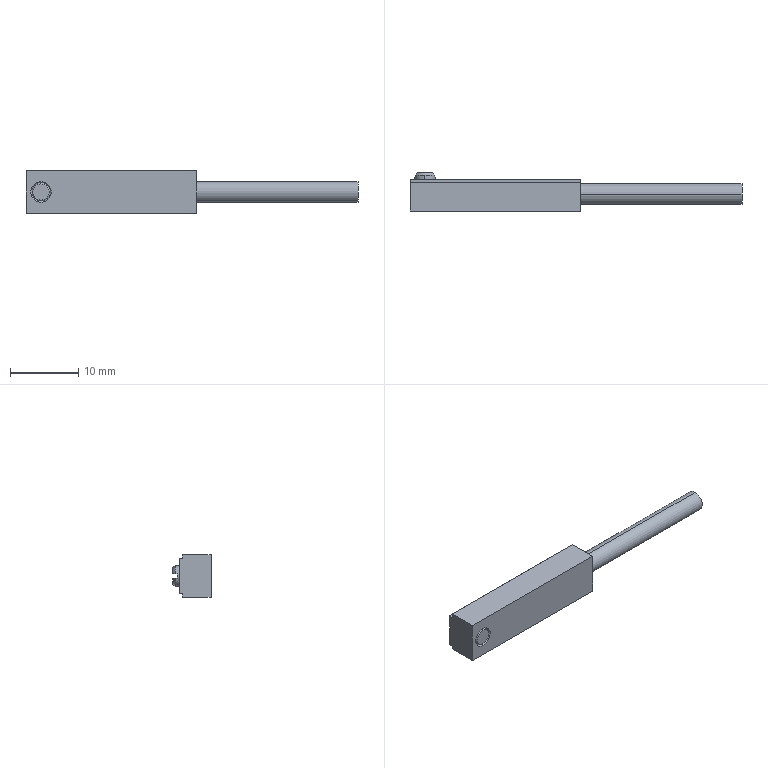Part | SolidWorks | features BaseBody 1 | 1 solid | 28 faces | box 48.8 x 5.6 x 6.3 mm | volume 899.301 mm3 | plane 17 | cone 7 | cylinder 4 | commonest cylinder face diameters 3 x4
STEP:
#1=CARTESIAN_POINT('',(0.7414,5.,-0.35));
#2=VERTEX_POINT('',#1);
#3=CARTESIAN_POINT('',(3.659,5.,-0.35));
#4=VERTEX_POINT('',#3);
#5=CARTESIAN_POINT('',(0.,5.,-0.35));
#6=DIRECTION('',(1.,0.,0.));
#7=VECTOR('',#6,1000.);
#8=LINE('',#5,#7);
#9=EDGE_CURVE('',#2,#4,#8,.T.);
#10=ORIENTED_EDGE('',*,*,#9,.F.);
#11=CARTESIAN_POINT('',(0.7414,5.,0.35));
#12=VERTEX_POINT('',#11);
#13=CARTESIAN_POINT('',(2.2,5.,0.));
#14=DIRECTION('',(0.,1.,0.));
#15=DIRECTION('',(0.,0.,1.));
#16=AXIS2_PLACEMENT_3D('',#13,#14,#15);
#17=CIRCLE('',#16,1.5);
#18=EDGE_CURVE('',#2,#12,#17,.T.);
#19=ORIENTED_EDGE('',*,*,#18,.T.);
#20=CARTESIAN_POINT('',(3.659,5.,0.35));
#21=VERTEX_POINT('',#20);
#22=CARTESIAN_POINT('',(0.,5.,0.35));
#23=DIRECTION('',(1.,0.,0.));
#24=VECTOR('',#23,1000.);
#25=LINE('',#22,#24);
#26=EDGE_CURVE('',#12,#21,#25,.T.);
#27=ORIENTED_EDGE('',*,*,#26,.T.);
#28=CARTESIAN_POINT('',(2.2,5.,0.));
#29=DIRECTION('',(0.,1.,0.));
#30=DIRECTION('',(0.,0.,1.));
#31=AXIS2_PLACEMENT_3D('',#28,#29,#30);
#32=CIRCLE('',#31,1.5);
#33=EDGE_CURVE('',#21,#4,#32,.T.);
#34=ORIENTED_EDGE('',*,*,#33,.T.);
#35=EDGE_LOOP('',(#10,#19,#27,#34));
#36=FACE_OUTER_BOUND('',#35,.T.);
#37=CARTESIAN_POINT('',(0.7,5.,0.35));
#38=DIRECTION('',(0.,1.,0.));
#39=DIRECTION('',(1.,0.,0.));
#40=AXIS2_PLACEMENT_3D('',#37,#38,#39);
#41=PLANE('',#40);
#42=ADVANCED_FACE('',(#36),#41,.T.);
#43=CARTESIAN_POINT('',(3.659,5.294,-0.35));
#44=VERTEX_POINT('',#43);
#45=CARTESIAN_POINT('',(3.341,5.6,-0.35));
#46=VERTEX_POINT('',#45);
#47=CARTESIAN_POINT('',(3.659,5.294,-0.35));
#48=CARTESIAN_POINT('',(3.553,5.396,-0.35));
#49=CARTESIAN_POINT('',(3.447,5.498,-0.35));
#50=CARTESIAN_POINT('',(3.341,5.6,-0.35));
#51=B_SPLINE_CURVE_WITH_KNOTS('',3,(#47,#48,#49,#50),.UNSPECIFIED.,.F.,.F.,(4,4),(0.,0.0004414),.UNSPECIFIED.);
#52=EDGE_CURVE('',#44,#46,#51,.T.);
#53=ORIENTED_EDGE('',*,*,#52,.T.);
#54=CARTESIAN_POINT('',(1.059,5.6,-0.35));
#55=VERTEX_POINT('',#54);
#56=CARTESIAN_POINT('',(2.2,5.6,-0.35));
#57=DIRECTION('',(-1.,0.,0.));
#58=VECTOR('',#57,1000.);
#59=LINE('',#56,#58);
#60=EDGE_CURVE('',#46,#55,#59,.T.);
#61=ORIENTED_EDGE('',*,*,#60,.T.);
#62=CARTESIAN_POINT('',(0.7414,5.294,-0.35));
#63=VERTEX_POINT('',#62);
#64=CARTESIAN_POINT('',(1.059,5.6,-0.35));
#65=CARTESIAN_POINT('',(0.9526,5.498,-0.35));
#66=CARTESIAN_POINT('',(0.8469,5.396,-0.35));
#67=CARTESIAN_POINT('',(0.7414,5.294,-0.35));
#68=B_SPLINE_CURVE_WITH_KNOTS('',3,(#64,#65,#66,#67),.UNSPECIFIED.,.F.,.F.,(4,4),(0.,0.0004414),.UNSPECIFIED.);
#69=EDGE_CURVE('',#55,#63,#68,.T.);
#70=ORIENTED_EDGE('',*,*,#69,.T.);
#71=CARTESIAN_POINT('',(0.7414,0.,-0.35));
#72=DIRECTION('',(0.,-1.,0.));
#73=VECTOR('',#72,1000.);
#74=LINE('',#71,#73);
#75=EDGE_CURVE('',#63,#2,#74,.T.);
#76=ORIENTED_EDGE('',*,*,#75,.T.);
#77=ORIENTED_EDGE('',*,*,#9,.T.);
#78=CARTESIAN_POINT('',(3.659,0.,-0.35));
#79=DIRECTION('',(0.,1.,0.));
#80=VECTOR('',#79,1000.);
#81=LINE('',#78,#80);
#82=EDGE_CURVE('',#4,#44,#81,.T.);
#83=ORIENTED_EDGE('',*,*,#82,.T.);
#84=EDGE_LOOP('',(#53,#61,#70,#76,#77,#83));
#85=FACE_OUTER_BOUND('',#84,.T.);
#86=CARTESIAN_POINT('',(0.,0.,-0.35));
#87=DIRECTION('',(0.,0.,1.));
#88=DIRECTION('',(1.,0.,0.));
#89=AXIS2_PLACEMENT_3D('',#86,#87,#88);
#90=PLANE('',#89);
#91=ADVANCED_FACE('',(#85),#90,.T.);
#92=CARTESIAN_POINT('',(3.659,5.294,0.35));
#93=VERTEX_POINT('',#92);
#94=CARTESIAN_POINT('',(3.341,5.6,0.35));
#95=VERTEX_POINT('',#94);
#96=CARTESIAN_POINT('',(3.659,5.294,0.35));
#97=CARTESIAN_POINT('',(3.553,5.396,0.35));
#98=CARTESIAN_POINT('',(3.447,5.498,0.35));
#99=CARTESIAN_POINT('',(3.341,5.6,0.35));
#100=B_SPLINE_CURVE_WITH_KNOTS('',3,(#96,#97,#98,#99),.UNSPECIFIED.,.F.,.F.,(4,4),(0.,0.0004414),.UNSPECIFIED.);
#101=EDGE_CURVE('',#93,#95,#100,.T.);
#102=ORIENTED_EDGE('',*,*,#101,.F.);
#103=CARTESIAN_POINT('',(3.659,0.,0.35));
#104=DIRECTION('',(0.,1.,0.));
#105=VECTOR('',#104,1000.);
#106=LINE('',#103,#105);
#107=EDGE_CURVE('',#21,#93,#106,.T.);
#108=ORIENTED_EDGE('',*,*,#107,.F.);
#109=ORIENTED_EDGE('',*,*,#26,.F.);
#110=CARTESIAN_POINT('',(0.7414,5.294,0.35));
#111=VERTEX_POINT('',#110);
#112=CARTESIAN_POINT('',(0.7414,0.,0.35));
#113=DIRECTION('',(0.,-1.,0.));
#114=VECTOR('',#113,1000.);
#115=LINE('',#112,#114);
#116=EDGE_CURVE('',#111,#12,#115,.T.);
#117=ORIENTED_EDGE('',*,*,#116,.F.);
#118=CARTESIAN_POINT('',(1.059,5.6,0.35));
#119=VERTEX_POINT('',#118);
#120=CARTESIAN_POINT('',(1.059,5.6,0.35));
#121=CARTESIAN_POINT('',(0.9526,5.498,0.35));
#122=CARTESIAN_POINT('',(0.8469,5.396,0.35));
#123=CARTESIAN_POINT('',(0.7414,5.294,0.35));
#124=B_SPLINE_CURVE_WITH_KNOTS('',3,(#120,#121,#122,#123),.UNSPECIFIED.,.F.,.F.,(4,4),(0.,0.0004414),.UNSPECIFIED.);
#125=EDGE_CURVE('',#119,#111,#124,.T.);
#126=ORIENTED_EDGE('',*,*,#125,.F.);
#127=CARTESIAN_POINT('',(2.2,5.6,0.35));
#128=DIRECTION('',(1.,0.,0.));
#129=VECTOR('',#128,1000.);
#130=LINE('',#127,#129);
#131=EDGE_CURVE('',#119,#95,#130,.T.);
#132=ORIENTED_EDGE('',*,*,#131,.T.);
#133=EDGE_LOOP('',(#102,#108,#109,#117,#126,#132));
#134=FACE_OUTER_BOUND('',#133,.T.);
#135=CARTESIAN_POINT('',(0.,0.,0.35));
#136=DIRECTION('',(0.,0.,1.));
#137=DIRECTION('',(1.,0.,0.));
#138=AXIS2_PLACEMENT_3D('',#135,#136,#137);
#139=PLANE('',#138);
#140=ADVANCED_FACE('',(#134),#139,.F.);
#141=CARTESIAN_POINT('',(2.2,0.,1.194));
#142=VERTEX_POINT('',#141);
#143=CARTESIAN_POINT('',(2.2,0.,-1.194));
#144=VERTEX_POINT('',#143);
#145=CARTESIAN_POINT('',(2.2,0.,0.));
#146=DIRECTION('',(0.,1.,0.));
#147=DIRECTION('',(0.,0.,1.));
#148=AXIS2_PLACEMENT_3D('',#145,#146,#147);
#149=CIRCLE('',#148,1.194);
#150=EDGE_CURVE('',#142,#144,#149,.T.);
#151=ORIENTED_EDGE('',*,*,#150,.F.);
#152=CARTESIAN_POINT('',(2.2,0.,0.));
#153=DIRECTION('',(0.,1.,0.));
#154=DIRECTION('',(0.,0.,1.));
#155=AXIS2_PLACEMENT_3D('',#152,#153,#154);
#156=CIRCLE('',#155,1.194);
#157=EDGE_CURVE('',#144,#142,#156,.T.);
#158=ORIENTED_EDGE('',*,*,#157,.F.);
#159=EDGE_LOOP('',(#151,#158));
#160=FACE_OUTER_BOUND('',#159,.T.);
#161=CARTESIAN_POINT('',(2.2,0.,-1.194));
#162=DIRECTION('',(0.,1.,0.));
#163=DIRECTION('',(1.,0.,0.));
#164=AXIS2_PLACEMENT_3D('',#161,#162,#163);
#165=PLANE('',#164);
#166=ADVANCED_FACE('',(#160),#165,.F.);
#167=CARTESIAN_POINT('',(2.2,5.6,-1.193));
#168=VERTEX_POINT('',#167);
#169=CARTESIAN_POINT('',(2.2,5.6,0.));
#170=DIRECTION('',(0.,-1.,0.));
#171=DIRECTION('',(0.,0.,-1.));
#172=AXIS2_PLACEMENT_3D('',#169,#170,#171);
#173=CIRCLE('',#172,1.193);
#174=EDGE_CURVE('',#55,#168,#173,.T.);
#175=ORIENTED_EDGE('',*,*,#174,.F.);
#176=ORIENTED_EDGE('',*,*,#60,.F.);
#177=CARTESIAN_POINT('',(2.2,5.6,0.));
#178=DIRECTION('',(0.,-1.,0.));
#179=DIRECTION('',(0.,0.,-1.));
#180=AXIS2_PLACEMENT_3D('',#177,#178,#179);
#181=CIRCLE('',#180,1.193);
#182=EDGE_CURVE('',#168,#46,#181,.T.);
#183=ORIENTED_EDGE('',*,*,#182,.F.);
#184=EDGE_LOOP('',(#175,#176,#183));
#185=FACE_OUTER_BOUND('',#184,.T.);
#186=CARTESIAN_POINT('',(2.2,5.6,0.));
#187=DIRECTION('',(0.,-1.,0.));
#188=DIRECTION('',(0.,0.,-1.));
#189=AXIS2_PLACEMENT_3D('',#186,#187,#188);
#190=PLANE('',#189);
#191=ADVANCED_FACE('',(#185),#190,.F.);
#192=ORIENTED_EDGE('',*,*,#131,.F.);
#193=CARTESIAN_POINT('',(2.2,5.6,0.));
#194=DIRECTION('',(0.,-1.,0.));
#195=DIRECTION('',(0.,0.,-1.));
#196=AXIS2_PLACEMENT_3D('',#193,#194,#195);
#197=CIRCLE('',#196,1.193);
#198=EDGE_CURVE('',#95,#119,#197,.T.);
#199=ORIENTED_EDGE('',*,*,#198,.F.);
#200=EDGE_LOOP('',(#192,#199));
#201=FACE_OUTER_BOUND('',#200,.T.);
#202=CARTESIAN_POINT('',(2.2,5.6,0.));
#203=DIRECTION('',(0.,-1.,0.));
#204=DIRECTION('',(0.,0.,-1.));
#205=AXIS2_PLACEMENT_3D('',#202,#203,#204);
#206=PLANE('',#205);
#207=ADVANCED_FACE('',(#201),#206,.F.);
#208=CARTESIAN_POINT('',(2.2,0.1532,-1.347));
#209=VERTEX_POINT('',#208);
#210=CARTESIAN_POINT('',(2.2,0.1532,-1.347));
#211=DIRECTION('',(0.,0.7071,-0.7071));
#212=VECTOR('',#211,1000.);
#213=LINE('',#210,#212);
#214=EDGE_CURVE('',#144,#209,#213,.T.);
#215=ORIENTED_EDGE('',*,*,#214,.F.);
#216=ORIENTED_EDGE('',*,*,#157,.T.);
#217=CARTESIAN_POINT('',(2.2,0.1532,1.347));
#218=VERTEX_POINT('',#217);
#219=CARTESIAN_POINT('',(2.2,0.1532,1.347));
#220=DIRECTION('',(0.,0.7071,0.7071));
#221=VECTOR('',#220,1000.);
#222=LINE('',#219,#221);
#223=EDGE_CURVE('',#142,#218,#222,.T.);
#224=ORIENTED_EDGE('',*,*,#223,.T.);
#225=CARTESIAN_POINT('',(2.2,0.1532,0.));
#226=DIRECTION('',(0.,-1.,0.));
#227=DIRECTION('',(0.,0.,-1.));
#228=AXIS2_PLACEMENT_3D('',#225,#226,#227);
#229=CIRCLE('',#228,1.347);
#230=EDGE_CURVE('',#218,#209,#229,.T.);
#231=ORIENTED_EDGE('',*,*,#230,.T.);
#232=EDGE_LOOP('',(#215,#216,#224,#231));
#233=FACE_OUTER_BOUND('',#232,.T.);
#234=CARTESIAN_POINT('',(2.2,0.1532,0.));
#235=DIRECTION('',(0.,1.,0.));
#236=DIRECTION('',(0.,0.,1.));
#237=AXIS2_PLACEMENT_3D('',#234,#235,#236);
#238=CONICAL_SURFACE('',#237,1.347,0.7854);
#239=ADVANCED_FACE('',(#233),#238,.T.);
#240=CARTESIAN_POINT('',(2.2,5.293,-1.5));
#241=VERTEX_POINT('',#240);
#242=CARTESIAN_POINT('',(2.2,5.294,-1.5));
#243=DIRECTION('',(0.,-0.7071,-0.7071));
#244=VECTOR('',#243,1000.);
#245=LINE('',#242,#244);
#246=EDGE_CURVE('',#168,#241,#245,.T.);
#247=ORIENTED_EDGE('',*,*,#246,.F.);
#248=ORIENTED_EDGE('',*,*,#182,.T.);
#249=ORIENTED_EDGE('',*,*,#52,.F.);
#250=CARTESIAN_POINT('',(2.2,5.293,0.));
#251=DIRECTION('',(0.,-1.,0.));
#252=DIRECTION('',(0.,0.,1.));
#253=AXIS2_PLACEMENT_3D('',#250,#251,#252);
#254=CIRCLE('',#253,1.5);
#255=EDGE_CURVE('',#241,#44,#254,.T.);
#256=ORIENTED_EDGE('',*,*,#255,.F.);
#257=EDGE_LOOP('',(#247,#248,#249,#256));
#258=FACE_OUTER_BOUND('',#257,.T.);
#259=CARTESIAN_POINT('',(2.2,5.294,0.));
#260=DIRECTION('',(0.,-1.,0.));
#261=DIRECTION('',(0.,0.,-1.));
#262=AXIS2_PLACEMENT_3D('',#259,#260,#261);
#263=CONICAL_SURFACE('',#262,1.5,0.7854);
#264=ADVANCED_FACE('',(#258),#263,.T.);
#265=ORIENTED_EDGE('',*,*,#198,.T.);
#266=ORIENTED_EDGE('',*,*,#125,.T.);
#267=CARTESIAN_POINT('',(2.2,5.293,1.5));
#268=VERTEX_POINT('',#267);
#269=CARTESIAN_POINT('',(2.2,5.293,0.));
#270=DIRECTION('',(0.,-1.,0.));
#271=DIRECTION('',(0.,0.,1.));
#272=AXIS2_PLACEMENT_3D('',#269,#270,#271);
#273=CIRCLE('',#272,1.5);
#274=EDGE_CURVE('',#268,#111,#273,.T.);
#275=ORIENTED_EDGE('',*,*,#274,.F.);
#276=CARTESIAN_POINT('',(2.2,5.293,0.));
#277=DIRECTION('',(0.,-1.,0.));
#278=DIRECTION('',(0.,0.,1.));
#279=AXIS2_PLACEMENT_3D('',#276,#277,#278);
#280=CIRCLE('',#279,1.5);
#281=EDGE_CURVE('',#93,#268,#280,.T.);
#282=ORIENTED_EDGE('',*,*,#281,.F.);
#283=ORIENTED_EDGE('',*,*,#101,.T.);
#284=EDGE_LOOP('',(#265,#266,#275,#282,#283));
#285=FACE_OUTER_BOUND('',#284,.T.);
#286=CARTESIAN_POINT('',(2.2,5.294,0.));
#287=DIRECTION('',(0.,-1.,0.));
#288=DIRECTION('',(0.,0.,-1.));
#289=AXIS2_PLACEMENT_3D('',#286,#287,#288);
#290=CONICAL_SURFACE('',#289,1.5,0.7854);
#291=ADVANCED_FACE('',(#285),#290,.T.);
#292=CARTESIAN_POINT('',(0.,4.2,3.15));
#293=VERTEX_POINT('',#292);
#294=CARTESIAN_POINT('',(25.,4.2,3.15));
#295=VERTEX_POINT('',#294);
#296=CARTESIAN_POINT('',(25.,4.2,3.15));
#297=DIRECTION('',(1.,0.,0.));
#298=VECTOR('',#297,1000.);
#299=LINE('',#296,#298);
#300=EDGE_CURVE('',#293,#295,#299,.T.);
#301=ORIENTED_EDGE('',*,*,#300,.T.);
#302=CARTESIAN_POINT('',(25.,4.2,2.6));
#303=VERTEX_POINT('',#302);
#304=CARTESIAN_POINT('',(25.,4.2,2.6));
#305=DIRECTION('',(0.,0.,1.));
#306=VECTOR('',#305,1000.);
#307=LINE('',#304,#306);
#308=EDGE_CURVE('',#303,#295,#307,.T.);
#309=ORIENTED_EDGE('',*,*,#308,.F.);
#310=CARTESIAN_POINT('',(0.,4.2,2.6));
#311=VERTEX_POINT('',#310);
#312=CARTESIAN_POINT('',(25.,4.2,2.6));
#313=DIRECTION('',(-1.,0.,0.));
#314=VECTOR('',#313,1000.);
#315=LINE('',#312,#314);
#316=EDGE_CURVE('',#303,#311,#315,.T.);
#317=ORIENTED_EDGE('',*,*,#316,.T.);
#318=CARTESIAN_POINT('',(0.,4.2,0.));
#319=DIRECTION('',(0.,0.,1.));
#320=VECTOR('',#319,1000.);
#321=LINE('',#318,#320);
#322=EDGE_CURVE('',#311,#293,#321,.T.);
#323=ORIENTED_EDGE('',*,*,#322,.T.);
#324=EDGE_LOOP('',(#301,#309,#317,#323));
#325=FACE_OUTER_BOUND('',#324,.T.);
#326=CARTESIAN_POINT('',(25.,4.2,2.6));
#327=DIRECTION('',(0.,-1.,0.));
#328=DIRECTION('',(0.,0.,-1.));
#329=AXIS2_PLACEMENT_3D('',#326,#327,#328);
#330=PLANE('',#329);
#331=ADVANCED_FACE('',(#325),#330,.F.);
#332=CARTESIAN_POINT('',(2.2,0.,1.5));
#333=VERTEX_POINT('',#332);
#334=CARTESIAN_POINT('',(2.2,0.,1.5));
#335=DIRECTION('',(0.,-0.7071,0.7071));
#336=VECTOR('',#335,1000.);
#337=LINE('',#334,#336);
#338=EDGE_CURVE('',#218,#333,#337,.T.);
#339=ORIENTED_EDGE('',*,*,#338,.F.);
#340=CARTESIAN_POINT('',(2.2,0.1532,0.));
#341=DIRECTION('',(0.,-1.,0.));
#342=DIRECTION('',(0.,0.,-1.));
#343=AXIS2_PLACEMENT_3D('',#340,#341,#342);
#344=CIRCLE('',#343,1.347);
#345=EDGE_CURVE('',#209,#218,#344,.T.);
#346=ORIENTED_EDGE('',*,*,#345,.F.);
#347=CARTESIAN_POINT('',(2.2,0.,-1.5));
#348=VERTEX_POINT('',#347);
#349=CARTESIAN_POINT('',(2.2,0.,-1.5));
#350=DIRECTION('',(0.,-0.7071,-0.7071));
#351=VECTOR('',#350,1000.);
#352=LINE('',#349,#351);
#353=EDGE_CURVE('',#209,#348,#352,.T.);
#354=ORIENTED_EDGE('',*,*,#353,.T.);
#355=CARTESIAN_POINT('',(2.2,0.,0.));
#356=DIRECTION('',(0.,-1.,0.));
#357=DIRECTION('',(0.,0.,-1.));
#358=AXIS2_PLACEMENT_3D('',#355,#356,#357);
#359=CIRCLE('',#358,1.5);
#360=EDGE_CURVE('',#348,#333,#359,.T.);
#361=ORIENTED_EDGE('',*,*,#360,.T.);
#362=EDGE_LOOP('',(#339,#346,#354,#361));
#363=FACE_OUTER_BOUND('',#362,.T.);
#364=CARTESIAN_POINT('',(2.2,0.,0.));
#365=DIRECTION('',(0.,-1.,0.));
#366=DIRECTION('',(0.,0.,-1.));
#367=AXIS2_PLACEMENT_3D('',#364,#365,#366);
#368=CONICAL_SURFACE('',#367,1.5,0.7854);
#369=ADVANCED_FACE('',(#363),#368,.F.);
#370=CARTESIAN_POINT('',(0.,4.2,-2.6));
#371=VERTEX_POINT('',#370);
#372=CARTESIAN_POINT('',(25.,4.2,-2.6));
#373=VERTEX_POINT('',#372);
#374=CARTESIAN_POINT('',(25.,4.2,-2.6));
#375=DIRECTION('',(1.,0.,0.));
#376=VECTOR('',#375,1000.);
#377=LINE('',#374,#376);
#378=EDGE_CURVE('',#371,#373,#377,.T.);
#379=ORIENTED_EDGE('',*,*,#378,.T.);
#380=CARTESIAN_POINT('',(25.,4.2,-3.15));
#381=VERTEX_POINT('',#380);
#382=CARTESIAN_POINT('',(25.,4.2,-3.15));
#383=DIRECTION('',(0.,0.,1.));
#384=VECTOR('',#383,1000.);
#385=LINE('',#382,#384);
#386=EDGE_CURVE('',#381,#373,#385,.T.);
#387=ORIENTED_EDGE('',*,*,#386,.F.);
#388=CARTESIAN_POINT('',(0.,4.2,-3.15));
#389=VERTEX_POINT('',#388);
#390=CARTESIAN_POINT('',(25.,4.2,-3.15));
#391=DIRECTION('',(-1.,0.,0.));
#392=VECTOR('',#391,1000.);
#393=LINE('',#390,#392);
#394=EDGE_CURVE('',#381,#389,#393,.T.);
#395=ORIENTED_EDGE('',*,*,#394,.T.);
#396=CARTESIAN_POINT('',(0.,4.2,0.));
#397=DIRECTION('',(0.,0.,1.));
#398=VECTOR('',#397,1000.);
#399=LINE('',#396,#398);
#400=EDGE_CURVE('',#389,#371,#399,.T.);
#401=ORIENTED_EDGE('',*,*,#400,.T.);
#402=EDGE_LOOP('',(#379,#387,#395,#401));
#403=FACE_OUTER_BOUND('',#402,.T.);
#404=CARTESIAN_POINT('',(25.,4.2,-3.15));
#405=DIRECTION('',(0.,-1.,0.));
#406=DIRECTION('',(0.,0.,-1.));
#407=AXIS2_PLACEMENT_3D('',#404,#405,#406);
#408=PLANE('',#407);
#409=ADVANCED_FACE('',(#403),#408,.F.);
#410=CARTESIAN_POINT('',(2.2,4.7,-1.5));
#411=VERTEX_POINT('',#410);
#412=CARTESIAN_POINT('',(2.2,0.,-1.5));
#413=DIRECTION('',(0.,1.,0.));
#414=VECTOR('',#413,1000.);
#415=LINE('',#412,#414);
#416=EDGE_CURVE('',#411,#241,#415,.T.);
#417=ORIENTED_EDGE('',*,*,#416,.F.);
#418=CARTESIAN_POINT('',(2.2,4.7,1.5));
#419=VERTEX_POINT('',#418);
#420=CARTESIAN_POINT('',(2.2,4.7,0.));
#421=DIRECTION('',(0.,1.,0.));
#422=DIRECTION('',(0.,0.,1.));
#423=AXIS2_PLACEMENT_3D('',#420,#421,#422);
#424=CIRCLE('',#423,1.5);
#425=EDGE_CURVE('',#411,#419,#424,.T.);
#426=ORIENTED_EDGE('',*,*,#425,.T.);
#427=CARTESIAN_POINT('',(2.2,0.,1.5));
#428=DIRECTION('',(0.,1.,0.));
#429=VECTOR('',#428,1000.);
#430=LINE('',#427,#429);
#431=EDGE_CURVE('',#419,#268,#430,.T.);
#432=ORIENTED_EDGE('',*,*,#431,.T.);
#433=ORIENTED_EDGE('',*,*,#274,.T.);
#434=ORIENTED_EDGE('',*,*,#116,.T.);
#435=ORIENTED_EDGE('',*,*,#18,.F.);
#436=ORIENTED_EDGE('',*,*,#75,.F.);
#437=CARTESIAN_POINT('',(2.2,5.293,0.));
#438=DIRECTION('',(0.,-1.,0.));
#439=DIRECTION('',(0.,0.,1.));
#440=AXIS2_PLACEMENT_3D('',#437,#438,#439);
#441=CIRCLE('',#440,1.5);
#442=EDGE_CURVE('',#63,#241,#441,.T.);
#443=ORIENTED_EDGE('',*,*,#442,.T.);
#444=EDGE_LOOP('',(#417,#426,#432,#433,#434,#435,#436,#443));
#445=FACE_OUTER_BOUND('',#444,.T.);
#446=CARTESIAN_POINT('',(2.2,0.,0.));
#447=DIRECTION('',(0.,1.,0.));
#448=DIRECTION('',(0.,0.,1.));
#449=AXIS2_PLACEMENT_3D('',#446,#447,#448);
#450=CYLINDRICAL_SURFACE('',#449,1.5);
#451=ADVANCED_FACE('',(#445),#450,.T.);
#452=CARTESIAN_POINT('',(0.,4.7,-2.6));
#453=VERTEX_POINT('',#452);
#454=CARTESIAN_POINT('',(25.,4.7,-2.6));
#455=VERTEX_POINT('',#454);
#456=CARTESIAN_POINT('',(25.,4.7,-2.6));
#457=DIRECTION('',(1.,0.,0.));
#458=VECTOR('',#457,1000.);
#459=LINE('',#456,#458);
#460=EDGE_CURVE('',#453,#455,#459,.T.);
#461=ORIENTED_EDGE('',*,*,#460,.T.);
#462=CARTESIAN_POINT('',(25.,4.2,-2.6));
#463=DIRECTION('',(0.,1.,0.));
#464=VECTOR('',#463,1000.);
#465=LINE('',#462,#464);
#466=EDGE_CURVE('',#373,#455,#465,.T.);
#467=ORIENTED_EDGE('',*,*,#466,.F.);
#468=ORIENTED_EDGE('',*,*,#378,.F.);
#469=CARTESIAN_POINT('',(0.,0.,-2.6));
#470=DIRECTION('',(0.,1.,0.));
#471=VECTOR('',#470,1000.);
#472=LINE('',#469,#471);
#473=EDGE_CURVE('',#371,#453,#472,.T.);
#474=ORIENTED_EDGE('',*,*,#473,.T.);
#475=EDGE_LOOP('',(#461,#467,#468,#474));
#476=FACE_OUTER_BOUND('',#475,.T.);
#477=CARTESIAN_POINT('',(25.,4.2,-2.6));
#478=DIRECTION('',(0.,0.,1.));
#479=DIRECTION('',(1.,0.,0.));
#480=AXIS2_PLACEMENT_3D('',#477,#478,#479);
#481=PLANE('',#480);
#482=ADVANCED_FACE('',(#476),#481,.F.);
#483=ORIENTED_EDGE('',*,*,#316,.F.);
#484=CARTESIAN_POINT('',(25.,4.7,2.6));
#485=VERTEX_POINT('',#484);
#486=CARTESIAN_POINT('',(25.,4.7,2.6));
#487=DIRECTION('',(0.,-1.,0.));
#488=VECTOR('',#487,1000.);
#489=LINE('',#486,#488);
#490=EDGE_CURVE('',#485,#303,#489,.T.);
#491=ORIENTED_EDGE('',*,*,#490,.F.);
#492=CARTESIAN_POINT('',(0.,4.7,2.6));
#493=VERTEX_POINT('',#492);
#494=CARTESIAN_POINT('',(25.,4.7,2.6));
#495=DIRECTION('',(-1.,0.,0.));
#496=VECTOR('',#495,1000.);
#497=LINE('',#494,#496);
#498=EDGE_CURVE('',#485,#493,#497,.T.);
#499=ORIENTED_EDGE('',*,*,#498,.T.);
#500=CARTESIAN_POINT('',(0.,0.,2.6));
#501=DIRECTION('',(0.,-1.,0.));
#502=VECTOR('',#501,1000.);
#503=LINE('',#500,#502);
#504=EDGE_CURVE('',#493,#311,#503,.T.);
#505=ORIENTED_EDGE('',*,*,#504,.T.);
#506=EDGE_LOOP('',(#483,#491,#499,#505));
#507=FACE_OUTER_BOUND('',#506,.T.);
#508=CARTESIAN_POINT('',(25.,4.7,2.6));
#509=DIRECTION('',(0.,0.,-1.));
#510=DIRECTION('',(0.,-1.,0.));
#511=AXIS2_PLACEMENT_3D('',#508,#509,#510);
#512=PLANE('',#511);
#513=ADVANCED_FACE('',(#507),#512,.F.);
#514=ORIENTED_EDGE('',*,*,#322,.F.);
#515=ORIENTED_EDGE('',*,*,#504,.F.);
#516=CARTESIAN_POINT('',(0.,4.7,-2.6));
#517=DIRECTION('',(0.,0.,-1.));
#518=VECTOR('',#517,1000.);
#519=LINE('',#516,#518);
#520=EDGE_CURVE('',#493,#453,#519,.T.);
#521=ORIENTED_EDGE('',*,*,#520,.T.);
#522=ORIENTED_EDGE('',*,*,#473,.F.);
#523=ORIENTED_EDGE('',*,*,#400,.F.);
#524=CARTESIAN_POINT('',(0.,0.,-3.15));
#525=VERTEX_POINT('',#524);
#526=CARTESIAN_POINT('',(0.,0.,-3.15));
#527=DIRECTION('',(0.,-1.,0.));
#528=VECTOR('',#527,1000.);
#529=LINE('',#526,#528);
#530=EDGE_CURVE('',#389,#525,#529,.T.);
#531=ORIENTED_EDGE('',*,*,#530,.T.);
#532=CARTESIAN_POINT('',(0.,0.,3.15));
#533=VERTEX_POINT('',#532);
#534=CARTESIAN_POINT('',(0.,0.,3.15));
#535=DIRECTION('',(0.,0.,1.));
#536=VECTOR('',#535,1000.);
#537=LINE('',#534,#536);
#538=EDGE_CURVE('',#525,#533,#537,.T.);
#539=ORIENTED_EDGE('',*,*,#538,.T.);
#540=CARTESIAN_POINT('',(0.,4.2,3.15));
#541=DIRECTION('',(0.,1.,0.));
#542=VECTOR('',#541,1000.);
#543=LINE('',#540,#542);
#544=EDGE_CURVE('',#533,#293,#543,.T.);
#545=ORIENTED_EDGE('',*,*,#544,.T.);
#546=EDGE_LOOP('',(#514,#515,#521,#522,#523,#531,#539,#545));
#547=FACE_OUTER_BOUND('',#546,.T.);
#548=CARTESIAN_POINT('',(0.,0.,0.));
#549=DIRECTION('',(1.,0.,0.));
#550=DIRECTION('',(0.,1.,0.));
#551=AXIS2_PLACEMENT_3D('',#548,#549,#550);
#552=PLANE('',#551);
#553=ADVANCED_FACE('',(#547),#552,.F.);
#554=CARTESIAN_POINT('',(25.,0.,3.15));
#555=VERTEX_POINT('',#554);
#556=CARTESIAN_POINT('',(25.,0.,3.15));
#557=DIRECTION('',(1.,0.,0.));
#558=VECTOR('',#557,1000.);
#559=LINE('',#556,#558);
#560=EDGE_CURVE('',#533,#555,#559,.T.);
#561=ORIENTED_EDGE('',*,*,#560,.T.);
#562=CARTESIAN_POINT('',(25.,0.,3.15));
#563=DIRECTION('',(0.,-1.,0.));
#564=VECTOR('',#563,1000.);
#565=LINE('',#562,#564);
#566=EDGE_CURVE('',#295,#555,#565,.T.);
#567=ORIENTED_EDGE('',*,*,#566,.F.);
#568=ORIENTED_EDGE('',*,*,#300,.F.);
#569=ORIENTED_EDGE('',*,*,#544,.F.);
#570=EDGE_LOOP('',(#561,#567,#568,#569));
#571=FACE_OUTER_BOUND('',#570,.T.);
#572=CARTESIAN_POINT('',(25.,4.2,3.15));
#573=DIRECTION('',(0.,0.,-1.));
#574=DIRECTION('',(0.,-1.,0.));
#575=AXIS2_PLACEMENT_3D('',#572,#573,#574);
#576=PLANE('',#575);
#577=ADVANCED_FACE('',(#571),#576,.F.);
#578=ORIENTED_EDGE('',*,*,#360,.F.);
#579=CARTESIAN_POINT('',(2.2,0.,0.));
#580=DIRECTION('',(0.,-1.,0.));
#581=DIRECTION('',(0.,0.,-1.));
#582=AXIS2_PLACEMENT_3D('',#579,#580,#581);
#583=CIRCLE('',#582,1.5);
#584=EDGE_CURVE('',#333,#348,#583,.T.);
#585=ORIENTED_EDGE('',*,*,#584,.F.);
#586=EDGE_LOOP('',(#578,#585));
#587=FACE_BOUND('',#586,.T.);
#588=CARTESIAN_POINT('',(25.,0.,-3.15));
#589=VERTEX_POINT('',#588);
#590=CARTESIAN_POINT('',(25.,0.,-3.15));
#591=DIRECTION('',(1.,0.,0.));
#592=VECTOR('',#591,1000.);
#593=LINE('',#590,#592);
#594=EDGE_CURVE('',#525,#589,#593,.T.);
#595=ORIENTED_EDGE('',*,*,#594,.T.);
#596=CARTESIAN_POINT('',(25.,0.,0.));
#597=DIRECTION('',(0.,0.,-1.));
#598=VECTOR('',#597,1000.);
#599=LINE('',#596,#598);
#600=EDGE_CURVE('',#555,#589,#599,.T.);
#601=ORIENTED_EDGE('',*,*,#600,.F.);
#602=ORIENTED_EDGE('',*,*,#560,.F.);
#603=ORIENTED_EDGE('',*,*,#538,.F.);
#604=EDGE_LOOP('',(#595,#601,#602,#603));
#605=FACE_OUTER_BOUND('',#604,.T.);
#606=CARTESIAN_POINT('',(25.,0.,3.15));
#607=DIRECTION('',(0.,1.,0.));
#608=DIRECTION('',(1.,0.,0.));
#609=AXIS2_PLACEMENT_3D('',#606,#607,#608);
#610=PLANE('',#609);
#611=ADVANCED_FACE('',(#587,#605),#610,.F.);
#612=ORIENTED_EDGE('',*,*,#394,.F.);
#613=CARTESIAN_POINT('',(25.,0.,-3.15));
#614=DIRECTION('',(0.,1.,0.));
#615=VECTOR('',#614,1000.);
#616=LINE('',#613,#615);
#617=EDGE_CURVE('',#589,#381,#616,.T.);
#618=ORIENTED_EDGE('',*,*,#617,.F.);
#619=ORIENTED_EDGE('',*,*,#594,.F.);
#620=ORIENTED_EDGE('',*,*,#530,.F.);
#621=EDGE_LOOP('',(#612,#618,#619,#620));
#622=FACE_OUTER_BOUND('',#621,.T.);
#623=CARTESIAN_POINT('',(25.,0.,-3.15));
#624=DIRECTION('',(0.,0.,1.));
#625=DIRECTION('',(1.,0.,0.));
#626=AXIS2_PLACEMENT_3D('',#623,#624,#625);
#627=PLANE('',#626);
#628=ADVANCED_FACE('',(#622),#627,.F.);
#629=CARTESIAN_POINT('',(2.2,4.7,0.));
#630=DIRECTION('',(0.,1.,0.));
#631=DIRECTION('',(0.,0.,1.));
#632=AXIS2_PLACEMENT_3D('',#629,#630,#631);
#633=CIRCLE('',#632,1.5);
#634=EDGE_CURVE('',#419,#411,#633,.T.);
#635=ORIENTED_EDGE('',*,*,#634,.F.);
#636=ORIENTED_EDGE('',*,*,#425,.F.);
#637=EDGE_LOOP('',(#635,#636));
#638=FACE_BOUND('',#637,.T.);
#639=ORIENTED_EDGE('',*,*,#498,.F.);
#640=CARTESIAN_POINT('',(25.,4.7,0.));
#641=DIRECTION('',(0.,0.,1.));
#642=VECTOR('',#641,1000.);
#643=LINE('',#640,#642);
#644=EDGE_CURVE('',#455,#485,#643,.T.);
#645=ORIENTED_EDGE('',*,*,#644,.F.);
#646=ORIENTED_EDGE('',*,*,#460,.F.);
#647=ORIENTED_EDGE('',*,*,#520,.F.);
#648=EDGE_LOOP('',(#639,#645,#646,#647));
#649=FACE_OUTER_BOUND('',#648,.T.);
#650=CARTESIAN_POINT('',(25.,4.7,-2.6));
#651=DIRECTION('',(0.,-1.,0.));
#652=DIRECTION('',(0.,0.,-1.));
#653=AXIS2_PLACEMENT_3D('',#650,#651,#652);
#654=PLANE('',#653);
#655=ADVANCED_FACE('',(#638,#649),#654,.F.);
#656=CARTESIAN_POINT('',(25.,2.5,-1.5));
#657=VERTEX_POINT('',#656);
#658=CARTESIAN_POINT('',(25.,2.5,1.5));
#659=VERTEX_POINT('',#658);
#660=CARTESIAN_POINT('',(25.,2.5,0.));
#661=DIRECTION('',(1.,0.,0.));
#662=DIRECTION('',(0.,0.,-1.));
#663=AXIS2_PLACEMENT_3D('',#660,#661,#662);
#664=CIRCLE('',#663,1.5);
#665=EDGE_CURVE('',#657,#659,#664,.T.);
#666=ORIENTED_EDGE('',*,*,#665,.F.);
#667=CARTESIAN_POINT('',(25.,2.5,0.));
#668=DIRECTION('',(1.,0.,0.));
#669=DIRECTION('',(0.,0.,-1.));
#670=AXIS2_PLACEMENT_3D('',#667,#668,#669);
#671=CIRCLE('',#670,1.5);
#672=EDGE_CURVE('',#659,#657,#671,.T.);
#673=ORIENTED_EDGE('',*,*,#672,.F.);
#674=EDGE_LOOP('',(#666,#673));
#675=FACE_BOUND('',#674,.T.);
#676=ORIENTED_EDGE('',*,*,#490,.T.);
#677=ORIENTED_EDGE('',*,*,#308,.T.);
#678=ORIENTED_EDGE('',*,*,#566,.T.);
#679=ORIENTED_EDGE('',*,*,#600,.T.);
#680=ORIENTED_EDGE('',*,*,#617,.T.);
#681=ORIENTED_EDGE('',*,*,#386,.T.);
#682=ORIENTED_EDGE('',*,*,#466,.T.);
#683=ORIENTED_EDGE('',*,*,#644,.T.);
#684=EDGE_LOOP('',(#676,#677,#678,#679,#680,#681,#682,#683));
#685=FACE_OUTER_BOUND('',#684,.T.);
#686=CARTESIAN_POINT('',(25.,0.,0.));
#687=DIRECTION('',(1.,0.,0.));
#688=DIRECTION('',(0.,1.,0.));
#689=AXIS2_PLACEMENT_3D('',#686,#687,#688);
#690=PLANE('',#689);
#691=ADVANCED_FACE('',(#675,#685),#690,.T.);
#692=CARTESIAN_POINT('',(48.8,2.5,-1.5));
#693=VERTEX_POINT('',#692);
#694=CARTESIAN_POINT('',(48.8,2.5,1.5));
#695=VERTEX_POINT('',#694);
#696=CARTESIAN_POINT('',(48.8,2.5,0.));
#697=DIRECTION('',(-1.,0.,0.));
#698=DIRECTION('',(0.,0.,-1.));
#699=AXIS2_PLACEMENT_3D('',#696,#697,#698);
#700=CIRCLE('',#699,1.5);
#701=EDGE_CURVE('',#693,#695,#700,.T.);
#702=ORIENTED_EDGE('',*,*,#701,.F.);
#703=CARTESIAN_POINT('',(48.8,2.5,0.));
#704=DIRECTION('',(-1.,0.,0.));
#705=DIRECTION('',(0.,0.,-1.));
#706=AXIS2_PLACEMENT_3D('',#703,#704,#705);
#707=CIRCLE('',#706,1.5);
#708=EDGE_CURVE('',#695,#693,#707,.T.);
#709=ORIENTED_EDGE('',*,*,#708,.F.);
#710=EDGE_LOOP('',(#702,#709));
#711=FACE_OUTER_BOUND('',#710,.T.);
#712=CARTESIAN_POINT('',(48.8,2.5,0.));
#713=DIRECTION('',(1.,0.,0.));
#714=DIRECTION('',(0.,1.,0.));
#715=AXIS2_PLACEMENT_3D('',#712,#713,#714);
#716=PLANE('',#715);
#717=ADVANCED_FACE('',(#711),#716,.T.);
#718=CARTESIAN_POINT('',(48.8,2.5,1.5));
#719=DIRECTION('',(1.,0.,0.));
#720=VECTOR('',#719,1000.);
#721=LINE('',#718,#720);
#722=EDGE_CURVE('',#659,#695,#721,.T.);
#723=ORIENTED_EDGE('',*,*,#722,.F.);
#724=ORIENTED_EDGE('',*,*,#672,.T.);
#725=CARTESIAN_POINT('',(48.8,2.5,-1.5));
#726=DIRECTION('',(1.,0.,0.));
#727=VECTOR('',#726,1000.);
#728=LINE('',#725,#727);
#729=EDGE_CURVE('',#657,#693,#728,.T.);
#730=ORIENTED_EDGE('',*,*,#729,.T.);
#731=ORIENTED_EDGE('',*,*,#701,.T.);
#732=EDGE_LOOP('',(#723,#724,#730,#731));
#733=FACE_OUTER_BOUND('',#732,.T.);
#734=CARTESIAN_POINT('',(48.8,2.5,0.));
#735=DIRECTION('',(1.,0.,0.));
#736=DIRECTION('',(0.,0.,-1.));
#737=AXIS2_PLACEMENT_3D('',#734,#735,#736);
#738=CYLINDRICAL_SURFACE('',#737,1.5);
#739=ADVANCED_FACE('',(#733),#738,.T.);
#740=ORIENTED_EDGE('',*,*,#150,.T.);
#741=ORIENTED_EDGE('',*,*,#214,.T.);
#742=ORIENTED_EDGE('',*,*,#345,.T.);
#743=ORIENTED_EDGE('',*,*,#223,.F.);
#744=EDGE_LOOP('',(#740,#741,#742,#743));
#745=FACE_OUTER_BOUND('',#744,.T.);
#746=CARTESIAN_POINT('',(2.2,0.1532,0.));
#747=DIRECTION('',(0.,1.,0.));
#748=DIRECTION('',(0.,0.,1.));
#749=AXIS2_PLACEMENT_3D('',#746,#747,#748);
#750=CONICAL_SURFACE('',#749,1.347,0.7854);
#751=ADVANCED_FACE('',(#745),#750,.T.);
#752=ORIENTED_EDGE('',*,*,#174,.T.);
#753=ORIENTED_EDGE('',*,*,#246,.T.);
#754=ORIENTED_EDGE('',*,*,#442,.F.);
#755=ORIENTED_EDGE('',*,*,#69,.F.);
#756=EDGE_LOOP('',(#752,#753,#754,#755));
#757=FACE_OUTER_BOUND('',#756,.T.);
#758=CARTESIAN_POINT('',(2.2,5.294,0.));
#759=DIRECTION('',(0.,-1.,0.));
#760=DIRECTION('',(0.,0.,-1.));
#761=AXIS2_PLACEMENT_3D('',#758,#759,#760);
#762=CONICAL_SURFACE('',#761,1.5,0.7854);
#763=ADVANCED_FACE('',(#757),#762,.T.);
#764=ORIENTED_EDGE('',*,*,#230,.F.);
#765=ORIENTED_EDGE('',*,*,#338,.T.);
#766=ORIENTED_EDGE('',*,*,#584,.T.);
#767=ORIENTED_EDGE('',*,*,#353,.F.);
#768=EDGE_LOOP('',(#764,#765,#766,#767));
#769=FACE_OUTER_BOUND('',#768,.T.);
#770=CARTESIAN_POINT('',(2.2,0.,0.));
#771=DIRECTION('',(0.,-1.,0.));
#772=DIRECTION('',(0.,0.,-1.));
#773=AXIS2_PLACEMENT_3D('',#770,#771,#772);
#774=CONICAL_SURFACE('',#773,1.5,0.7854);
#775=ADVANCED_FACE('',(#769),#774,.F.);
#776=ORIENTED_EDGE('',*,*,#634,.T.);
#777=ORIENTED_EDGE('',*,*,#416,.T.);
#778=ORIENTED_EDGE('',*,*,#255,.T.);
#779=ORIENTED_EDGE('',*,*,#82,.F.);
#780=ORIENTED_EDGE('',*,*,#33,.F.);
#781=ORIENTED_EDGE('',*,*,#107,.T.);
#782=ORIENTED_EDGE('',*,*,#281,.T.);
#783=ORIENTED_EDGE('',*,*,#431,.F.);
#784=EDGE_LOOP('',(#776,#777,#778,#779,#780,#781,#782,#783));
#785=FACE_OUTER_BOUND('',#784,.T.);
#786=CARTESIAN_POINT('',(2.2,0.,0.));
#787=DIRECTION('',(0.,1.,0.));
#788=DIRECTION('',(0.,0.,1.));
#789=AXIS2_PLACEMENT_3D('',#786,#787,#788);
#790=CYLINDRICAL_SURFACE('',#789,1.5);
#791=ADVANCED_FACE('',(#785),#790,.T.);
#792=ORIENTED_EDGE('',*,*,#665,.T.);
#793=ORIENTED_EDGE('',*,*,#722,.T.);
#794=ORIENTED_EDGE('',*,*,#708,.T.);
#795=ORIENTED_EDGE('',*,*,#729,.F.);
#796=EDGE_LOOP('',(#792,#793,#794,#795));
#797=FACE_OUTER_BOUND('',#796,.T.);
#798=CARTESIAN_POINT('',(48.8,2.5,0.));
#799=DIRECTION('',(1.,0.,0.));
#800=DIRECTION('',(0.,0.,-1.));
#801=AXIS2_PLACEMENT_3D('',#798,#799,#800);
#802=CYLINDRICAL_SURFACE('',#801,1.5);
#803=ADVANCED_FACE('',(#797),#802,.T.);
#804=CLOSED_SHELL('',(#42,#91,#140,#166,#191,#207,#239,#264,#291,#331,#369,#409,#451,#482,#513,#553,#577,#611,#628,#655,#691,#717,#739,#751,#763,#775,#791,#803));
#805=MANIFOLD_SOLID_BREP('',#804);
#806=CARTESIAN_POINT('',(0.,0.,0.));
#807=DIRECTION('',(0.,0.,1.));
#808=DIRECTION('',(1.,0.,0.));
#809=AXIS2_PLACEMENT_3D('',#806,#807,#808);
#810=(LENGTH_UNIT()NAMED_UNIT(*)SI_UNIT(.MILLI.,.METRE.));
#811=UNCERTAINTY_MEASURE_WITH_UNIT(LENGTH_MEASURE(0.00001),#810,'','');
#812=(NAMED_UNIT(*)PLANE_ANGLE_UNIT()SI_UNIT($,.RADIAN.));
#813=(NAMED_UNIT(*)SI_UNIT($,.STERADIAN.)SOLID_ANGLE_UNIT());
#814=(GEOMETRIC_REPRESENTATION_CONTEXT(3)GLOBAL_UNCERTAINTY_ASSIGNED_CONTEXT((#811))GLOBAL_UNIT_ASSIGNED_CONTEXT((#810,#812,#813))REPRESENTATION_CONTEXT('',''));
#815=ADVANCED_BREP_SHAPE_REPRESENTATION('',(#805,#809),#814);